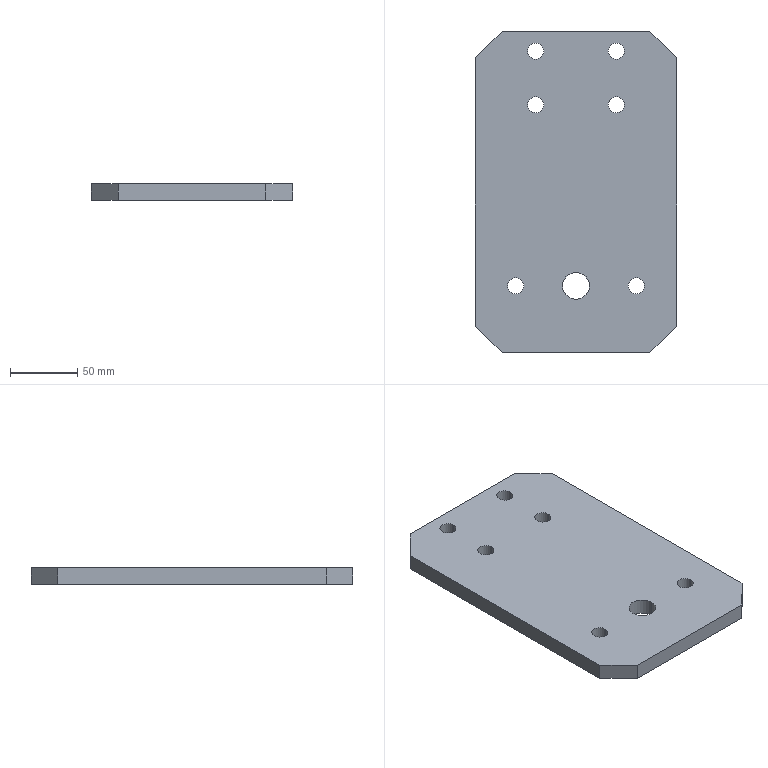Part | STEP file | Connecting plate | 1 solid | 24 faces | box 150 x 240 x 12 mm | volume 410487 mm3 | cylinder 14 | plane 10 | commonest cylinder face diameters 12 x12 20 x2
STEP:
#1=CARTESIAN_POINT('',(-24.923,-107.441,12.));
#2=VERTEX_POINT('',#1);
#3=CARTESIAN_POINT('',(-36.923,-107.441,12.));
#4=VERTEX_POINT('',#3);
#5=CARTESIAN_POINT('',(-30.923,-107.441,12.));
#6=DIRECTION('',(0.,0.,-1.));
#7=DIRECTION('',(-1.,0.,0.));
#8=AXIS2_PLACEMENT_3D('',#5,#6,#7);
#9=CIRCLE('',#8,6.);
#10=EDGE_CURVE('',#2,#4,#9,.T.);
#11=ORIENTED_EDGE('',*,*,#10,.F.);
#12=CARTESIAN_POINT('',(-24.923,-107.441,0.));
#13=VERTEX_POINT('',#12);
#14=CARTESIAN_POINT('',(-24.923,-107.441,12.));
#15=DIRECTION('',(0.,0.,-1.));
#16=VECTOR('',#15,1000.);
#17=LINE('',#14,#16);
#18=EDGE_CURVE('',#2,#13,#17,.T.);
#19=ORIENTED_EDGE('',*,*,#18,.T.);
#20=CARTESIAN_POINT('',(-36.923,-107.441,0.));
#21=VERTEX_POINT('',#20);
#22=CARTESIAN_POINT('',(-30.923,-107.441,0.));
#23=DIRECTION('',(0.,0.,-1.));
#24=DIRECTION('',(-1.,0.,0.));
#25=AXIS2_PLACEMENT_3D('',#22,#23,#24);
#26=CIRCLE('',#25,6.);
#27=EDGE_CURVE('',#13,#21,#26,.T.);
#28=ORIENTED_EDGE('',*,*,#27,.T.);
#29=CARTESIAN_POINT('',(-36.923,-107.441,12.));
#30=DIRECTION('',(0.,0.,-1.));
#31=VECTOR('',#30,1000.);
#32=LINE('',#29,#31);
#33=EDGE_CURVE('',#4,#21,#32,.T.);
#34=ORIENTED_EDGE('',*,*,#33,.F.);
#35=EDGE_LOOP('',(#11,#19,#28,#34));
#36=FACE_OUTER_BOUND('',#35,.T.);
#37=CARTESIAN_POINT('',(-30.923,-107.441,12.));
#38=DIRECTION('',(0.,0.,-1.));
#39=DIRECTION('',(-1.,0.,0.));
#40=AXIS2_PLACEMENT_3D('',#37,#38,#39);
#41=CYLINDRICAL_SURFACE('',#40,6.);
#42=ADVANCED_FACE('',(#36),#41,.F.);
#43=CARTESIAN_POINT('',(24.077,-107.441,12.));
#44=VERTEX_POINT('',#43);
#45=CARTESIAN_POINT('',(4.077,-107.441,12.));
#46=VERTEX_POINT('',#45);
#47=CARTESIAN_POINT('',(14.077,-107.441,12.));
#48=DIRECTION('',(0.,0.,-1.));
#49=DIRECTION('',(-1.,0.,0.));
#50=AXIS2_PLACEMENT_3D('',#47,#48,#49);
#51=CIRCLE('',#50,10.);
#52=EDGE_CURVE('',#44,#46,#51,.T.);
#53=ORIENTED_EDGE('',*,*,#52,.F.);
#54=CARTESIAN_POINT('',(24.077,-107.441,0.));
#55=VERTEX_POINT('',#54);
#56=CARTESIAN_POINT('',(24.077,-107.441,12.));
#57=DIRECTION('',(0.,0.,-1.));
#58=VECTOR('',#57,1000.);
#59=LINE('',#56,#58);
#60=EDGE_CURVE('',#44,#55,#59,.T.);
#61=ORIENTED_EDGE('',*,*,#60,.T.);
#62=CARTESIAN_POINT('',(4.077,-107.441,0.));
#63=VERTEX_POINT('',#62);
#64=CARTESIAN_POINT('',(14.077,-107.441,0.));
#65=DIRECTION('',(0.,0.,-1.));
#66=DIRECTION('',(-1.,0.,0.));
#67=AXIS2_PLACEMENT_3D('',#64,#65,#66);
#68=CIRCLE('',#67,10.);
#69=EDGE_CURVE('',#55,#63,#68,.T.);
#70=ORIENTED_EDGE('',*,*,#69,.T.);
#71=CARTESIAN_POINT('',(4.077,-107.441,12.));
#72=DIRECTION('',(0.,0.,-1.));
#73=VECTOR('',#72,1000.);
#74=LINE('',#71,#73);
#75=EDGE_CURVE('',#46,#63,#74,.T.);
#76=ORIENTED_EDGE('',*,*,#75,.F.);
#77=EDGE_LOOP('',(#53,#61,#70,#76));
#78=FACE_OUTER_BOUND('',#77,.T.);
#79=CARTESIAN_POINT('',(14.077,-107.441,12.));
#80=DIRECTION('',(0.,0.,-1.));
#81=DIRECTION('',(-1.,0.,0.));
#82=AXIS2_PLACEMENT_3D('',#79,#80,#81);
#83=CYLINDRICAL_SURFACE('',#82,10.);
#84=ADVANCED_FACE('',(#78),#83,.F.);
#85=CARTESIAN_POINT('',(50.077,27.559,12.));
#86=VERTEX_POINT('',#85);
#87=CARTESIAN_POINT('',(38.077,27.559,12.));
#88=VERTEX_POINT('',#87);
#89=CARTESIAN_POINT('',(44.077,27.559,12.));
#90=DIRECTION('',(0.,0.,-1.));
#91=DIRECTION('',(-1.,0.,0.));
#92=AXIS2_PLACEMENT_3D('',#89,#90,#91);
#93=CIRCLE('',#92,6.);
#94=EDGE_CURVE('',#86,#88,#93,.T.);
#95=ORIENTED_EDGE('',*,*,#94,.F.);
#96=CARTESIAN_POINT('',(50.077,27.559,0.));
#97=VERTEX_POINT('',#96);
#98=CARTESIAN_POINT('',(50.077,27.559,12.));
#99=DIRECTION('',(0.,0.,-1.));
#100=VECTOR('',#99,1000.);
#101=LINE('',#98,#100);
#102=EDGE_CURVE('',#86,#97,#101,.T.);
#103=ORIENTED_EDGE('',*,*,#102,.T.);
#104=CARTESIAN_POINT('',(38.077,27.559,0.));
#105=VERTEX_POINT('',#104);
#106=CARTESIAN_POINT('',(44.077,27.559,0.));
#107=DIRECTION('',(0.,0.,-1.));
#108=DIRECTION('',(-1.,0.,0.));
#109=AXIS2_PLACEMENT_3D('',#106,#107,#108);
#110=CIRCLE('',#109,6.);
#111=EDGE_CURVE('',#97,#105,#110,.T.);
#112=ORIENTED_EDGE('',*,*,#111,.T.);
#113=CARTESIAN_POINT('',(38.077,27.559,12.));
#114=DIRECTION('',(0.,0.,-1.));
#115=VECTOR('',#114,1000.);
#116=LINE('',#113,#115);
#117=EDGE_CURVE('',#88,#105,#116,.T.);
#118=ORIENTED_EDGE('',*,*,#117,.F.);
#119=EDGE_LOOP('',(#95,#103,#112,#118));
#120=FACE_OUTER_BOUND('',#119,.T.);
#121=CARTESIAN_POINT('',(44.077,27.559,12.));
#122=DIRECTION('',(0.,0.,-1.));
#123=DIRECTION('',(-1.,0.,0.));
#124=AXIS2_PLACEMENT_3D('',#121,#122,#123);
#125=CYLINDRICAL_SURFACE('',#124,6.);
#126=ADVANCED_FACE('',(#120),#125,.F.);
#127=CARTESIAN_POINT('',(-9.923,67.559,12.));
#128=VERTEX_POINT('',#127);
#129=CARTESIAN_POINT('',(-21.923,67.559,12.));
#130=VERTEX_POINT('',#129);
#131=CARTESIAN_POINT('',(-15.923,67.559,12.));
#132=DIRECTION('',(0.,0.,-1.));
#133=DIRECTION('',(-1.,0.,0.));
#134=AXIS2_PLACEMENT_3D('',#131,#132,#133);
#135=CIRCLE('',#134,6.);
#136=EDGE_CURVE('',#128,#130,#135,.T.);
#137=ORIENTED_EDGE('',*,*,#136,.F.);
#138=CARTESIAN_POINT('',(-9.923,67.559,0.));
#139=VERTEX_POINT('',#138);
#140=CARTESIAN_POINT('',(-9.923,67.559,12.));
#141=DIRECTION('',(0.,0.,-1.));
#142=VECTOR('',#141,1000.);
#143=LINE('',#140,#142);
#144=EDGE_CURVE('',#128,#139,#143,.T.);
#145=ORIENTED_EDGE('',*,*,#144,.T.);
#146=CARTESIAN_POINT('',(-21.923,67.559,0.));
#147=VERTEX_POINT('',#146);
#148=CARTESIAN_POINT('',(-15.923,67.559,0.));
#149=DIRECTION('',(0.,0.,-1.));
#150=DIRECTION('',(-1.,0.,0.));
#151=AXIS2_PLACEMENT_3D('',#148,#149,#150);
#152=CIRCLE('',#151,6.);
#153=EDGE_CURVE('',#139,#147,#152,.T.);
#154=ORIENTED_EDGE('',*,*,#153,.T.);
#155=CARTESIAN_POINT('',(-21.923,67.559,12.));
#156=DIRECTION('',(0.,0.,-1.));
#157=VECTOR('',#156,1000.);
#158=LINE('',#155,#157);
#159=EDGE_CURVE('',#130,#147,#158,.T.);
#160=ORIENTED_EDGE('',*,*,#159,.F.);
#161=EDGE_LOOP('',(#137,#145,#154,#160));
#162=FACE_OUTER_BOUND('',#161,.T.);
#163=CARTESIAN_POINT('',(-15.923,67.559,12.));
#164=DIRECTION('',(0.,0.,-1.));
#165=DIRECTION('',(-1.,0.,0.));
#166=AXIS2_PLACEMENT_3D('',#163,#164,#165);
#167=CYLINDRICAL_SURFACE('',#166,6.);
#168=ADVANCED_FACE('',(#162),#167,.F.);
#169=CARTESIAN_POINT('',(50.077,67.559,12.));
#170=VERTEX_POINT('',#169);
#171=CARTESIAN_POINT('',(38.077,67.559,12.));
#172=VERTEX_POINT('',#171);
#173=CARTESIAN_POINT('',(44.077,67.559,12.));
#174=DIRECTION('',(0.,0.,-1.));
#175=DIRECTION('',(-1.,0.,0.));
#176=AXIS2_PLACEMENT_3D('',#173,#174,#175);
#177=CIRCLE('',#176,6.);
#178=EDGE_CURVE('',#170,#172,#177,.T.);
#179=ORIENTED_EDGE('',*,*,#178,.F.);
#180=CARTESIAN_POINT('',(50.077,67.559,0.));
#181=VERTEX_POINT('',#180);
#182=CARTESIAN_POINT('',(50.077,67.559,12.));
#183=DIRECTION('',(0.,0.,-1.));
#184=VECTOR('',#183,1000.);
#185=LINE('',#182,#184);
#186=EDGE_CURVE('',#170,#181,#185,.T.);
#187=ORIENTED_EDGE('',*,*,#186,.T.);
#188=CARTESIAN_POINT('',(38.077,67.559,0.));
#189=VERTEX_POINT('',#188);
#190=CARTESIAN_POINT('',(44.077,67.559,0.));
#191=DIRECTION('',(0.,0.,-1.));
#192=DIRECTION('',(-1.,0.,0.));
#193=AXIS2_PLACEMENT_3D('',#190,#191,#192);
#194=CIRCLE('',#193,6.);
#195=EDGE_CURVE('',#181,#189,#194,.T.);
#196=ORIENTED_EDGE('',*,*,#195,.T.);
#197=CARTESIAN_POINT('',(38.077,67.559,12.));
#198=DIRECTION('',(0.,0.,-1.));
#199=VECTOR('',#198,1000.);
#200=LINE('',#197,#199);
#201=EDGE_CURVE('',#172,#189,#200,.T.);
#202=ORIENTED_EDGE('',*,*,#201,.F.);
#203=EDGE_LOOP('',(#179,#187,#196,#202));
#204=FACE_OUTER_BOUND('',#203,.T.);
#205=CARTESIAN_POINT('',(44.077,67.559,12.));
#206=DIRECTION('',(0.,0.,-1.));
#207=DIRECTION('',(-1.,0.,0.));
#208=AXIS2_PLACEMENT_3D('',#205,#206,#207);
#209=CYLINDRICAL_SURFACE('',#208,6.);
#210=ADVANCED_FACE('',(#204),#209,.F.);
#211=CARTESIAN_POINT('',(-9.923,27.559,12.));
#212=VERTEX_POINT('',#211);
#213=CARTESIAN_POINT('',(-21.923,27.559,12.));
#214=VERTEX_POINT('',#213);
#215=CARTESIAN_POINT('',(-15.923,27.559,12.));
#216=DIRECTION('',(0.,0.,-1.));
#217=DIRECTION('',(-1.,0.,0.));
#218=AXIS2_PLACEMENT_3D('',#215,#216,#217);
#219=CIRCLE('',#218,6.);
#220=EDGE_CURVE('',#212,#214,#219,.T.);
#221=ORIENTED_EDGE('',*,*,#220,.F.);
#222=CARTESIAN_POINT('',(-9.923,27.559,0.));
#223=VERTEX_POINT('',#222);
#224=CARTESIAN_POINT('',(-9.923,27.559,12.));
#225=DIRECTION('',(0.,0.,-1.));
#226=VECTOR('',#225,1000.);
#227=LINE('',#224,#226);
#228=EDGE_CURVE('',#212,#223,#227,.T.);
#229=ORIENTED_EDGE('',*,*,#228,.T.);
#230=CARTESIAN_POINT('',(-21.923,27.559,0.));
#231=VERTEX_POINT('',#230);
#232=CARTESIAN_POINT('',(-15.923,27.559,0.));
#233=DIRECTION('',(0.,0.,-1.));
#234=DIRECTION('',(-1.,0.,0.));
#235=AXIS2_PLACEMENT_3D('',#232,#233,#234);
#236=CIRCLE('',#235,6.);
#237=EDGE_CURVE('',#223,#231,#236,.T.);
#238=ORIENTED_EDGE('',*,*,#237,.T.);
#239=CARTESIAN_POINT('',(-21.923,27.559,12.));
#240=DIRECTION('',(0.,0.,-1.));
#241=VECTOR('',#240,1000.);
#242=LINE('',#239,#241);
#243=EDGE_CURVE('',#214,#231,#242,.T.);
#244=ORIENTED_EDGE('',*,*,#243,.F.);
#245=EDGE_LOOP('',(#221,#229,#238,#244));
#246=FACE_OUTER_BOUND('',#245,.T.);
#247=CARTESIAN_POINT('',(-15.923,27.559,12.));
#248=DIRECTION('',(0.,0.,-1.));
#249=DIRECTION('',(-1.,0.,0.));
#250=AXIS2_PLACEMENT_3D('',#247,#248,#249);
#251=CYLINDRICAL_SURFACE('',#250,6.);
#252=ADVANCED_FACE('',(#246),#251,.F.);
#253=CARTESIAN_POINT('',(65.077,-107.441,12.));
#254=VERTEX_POINT('',#253);
#255=CARTESIAN_POINT('',(53.077,-107.441,12.));
#256=VERTEX_POINT('',#255);
#257=CARTESIAN_POINT('',(59.077,-107.441,12.));
#258=DIRECTION('',(0.,0.,-1.));
#259=DIRECTION('',(-1.,0.,0.));
#260=AXIS2_PLACEMENT_3D('',#257,#258,#259);
#261=CIRCLE('',#260,6.);
#262=EDGE_CURVE('',#254,#256,#261,.T.);
#263=ORIENTED_EDGE('',*,*,#262,.F.);
#264=CARTESIAN_POINT('',(65.077,-107.441,0.));
#265=VERTEX_POINT('',#264);
#266=CARTESIAN_POINT('',(65.077,-107.441,12.));
#267=DIRECTION('',(0.,0.,-1.));
#268=VECTOR('',#267,1000.);
#269=LINE('',#266,#268);
#270=EDGE_CURVE('',#254,#265,#269,.T.);
#271=ORIENTED_EDGE('',*,*,#270,.T.);
#272=CARTESIAN_POINT('',(53.077,-107.441,0.));
#273=VERTEX_POINT('',#272);
#274=CARTESIAN_POINT('',(59.077,-107.441,0.));
#275=DIRECTION('',(0.,0.,-1.));
#276=DIRECTION('',(-1.,0.,0.));
#277=AXIS2_PLACEMENT_3D('',#274,#275,#276);
#278=CIRCLE('',#277,6.);
#279=EDGE_CURVE('',#265,#273,#278,.T.);
#280=ORIENTED_EDGE('',*,*,#279,.T.);
#281=CARTESIAN_POINT('',(53.077,-107.441,12.));
#282=DIRECTION('',(0.,0.,-1.));
#283=VECTOR('',#282,1000.);
#284=LINE('',#281,#283);
#285=EDGE_CURVE('',#256,#273,#284,.T.);
#286=ORIENTED_EDGE('',*,*,#285,.F.);
#287=EDGE_LOOP('',(#263,#271,#280,#286));
#288=FACE_OUTER_BOUND('',#287,.T.);
#289=CARTESIAN_POINT('',(59.077,-107.441,12.));
#290=DIRECTION('',(0.,0.,-1.));
#291=DIRECTION('',(-1.,0.,0.));
#292=AXIS2_PLACEMENT_3D('',#289,#290,#291);
#293=CYLINDRICAL_SURFACE('',#292,6.);
#294=ADVANCED_FACE('',(#288),#293,.F.);
#295=CARTESIAN_POINT('',(-30.923,-107.441,0.));
#296=DIRECTION('',(0.,0.,-1.));
#297=DIRECTION('',(-1.,0.,0.));
#298=AXIS2_PLACEMENT_3D('',#295,#296,#297);
#299=CIRCLE('',#298,6.);
#300=EDGE_CURVE('',#21,#13,#299,.T.);
#301=ORIENTED_EDGE('',*,*,#300,.F.);
#302=ORIENTED_EDGE('',*,*,#27,.F.);
#303=EDGE_LOOP('',(#301,#302));
#304=FACE_BOUND('',#303,.T.);
#305=CARTESIAN_POINT('',(14.077,-107.441,0.));
#306=DIRECTION('',(0.,0.,-1.));
#307=DIRECTION('',(-1.,0.,0.));
#308=AXIS2_PLACEMENT_3D('',#305,#306,#307);
#309=CIRCLE('',#308,10.);
#310=EDGE_CURVE('',#63,#55,#309,.T.);
#311=ORIENTED_EDGE('',*,*,#310,.F.);
#312=ORIENTED_EDGE('',*,*,#69,.F.);
#313=EDGE_LOOP('',(#311,#312));
#314=FACE_BOUND('',#313,.T.);
#315=CARTESIAN_POINT('',(44.077,27.559,0.));
#316=DIRECTION('',(0.,0.,-1.));
#317=DIRECTION('',(-1.,0.,0.));
#318=AXIS2_PLACEMENT_3D('',#315,#316,#317);
#319=CIRCLE('',#318,6.);
#320=EDGE_CURVE('',#105,#97,#319,.T.);
#321=ORIENTED_EDGE('',*,*,#320,.F.);
#322=ORIENTED_EDGE('',*,*,#111,.F.);
#323=EDGE_LOOP('',(#321,#322));
#324=FACE_BOUND('',#323,.T.);
#325=CARTESIAN_POINT('',(-15.923,67.559,0.));
#326=DIRECTION('',(0.,0.,-1.));
#327=DIRECTION('',(-1.,0.,0.));
#328=AXIS2_PLACEMENT_3D('',#325,#326,#327);
#329=CIRCLE('',#328,6.);
#330=EDGE_CURVE('',#147,#139,#329,.T.);
#331=ORIENTED_EDGE('',*,*,#330,.F.);
#332=ORIENTED_EDGE('',*,*,#153,.F.);
#333=EDGE_LOOP('',(#331,#332));
#334=FACE_BOUND('',#333,.T.);
#335=CARTESIAN_POINT('',(89.077,62.559,0.));
#336=VERTEX_POINT('',#335);
#337=CARTESIAN_POINT('',(69.077,82.559,0.));
#338=VERTEX_POINT('',#337);
#339=CARTESIAN_POINT('',(89.077,62.559,0.));
#340=DIRECTION('',(-0.7071,0.7071,0.));
#341=VECTOR('',#340,1000.);
#342=LINE('',#339,#341);
#343=EDGE_CURVE('',#336,#338,#342,.T.);
#344=ORIENTED_EDGE('',*,*,#343,.F.);
#345=CARTESIAN_POINT('',(89.077,-137.441,0.));
#346=VERTEX_POINT('',#345);
#347=CARTESIAN_POINT('',(89.077,-157.441,0.));
#348=DIRECTION('',(0.,1.,0.));
#349=VECTOR('',#348,1000.);
#350=LINE('',#347,#349);
#351=EDGE_CURVE('',#346,#336,#350,.T.);
#352=ORIENTED_EDGE('',*,*,#351,.F.);
#353=CARTESIAN_POINT('',(69.077,-157.441,0.));
#354=VERTEX_POINT('',#353);
#355=CARTESIAN_POINT('',(69.077,-157.441,0.));
#356=DIRECTION('',(0.7071,0.7071,0.));
#357=VECTOR('',#356,1000.);
#358=LINE('',#355,#357);
#359=EDGE_CURVE('',#354,#346,#358,.T.);
#360=ORIENTED_EDGE('',*,*,#359,.F.);
#361=CARTESIAN_POINT('',(-40.923,-157.441,0.));
#362=VERTEX_POINT('',#361);
#363=CARTESIAN_POINT('',(-60.923,-157.441,0.));
#364=DIRECTION('',(1.,0.,0.));
#365=VECTOR('',#364,1000.);
#366=LINE('',#363,#365);
#367=EDGE_CURVE('',#362,#354,#366,.T.);
#368=ORIENTED_EDGE('',*,*,#367,.F.);
#369=CARTESIAN_POINT('',(-60.923,-137.441,0.));
#370=VERTEX_POINT('',#369);
#371=CARTESIAN_POINT('',(-60.923,-137.441,0.));
#372=DIRECTION('',(0.7071,-0.7071,0.));
#373=VECTOR('',#372,1000.);
#374=LINE('',#371,#373);
#375=EDGE_CURVE('',#370,#362,#374,.T.);
#376=ORIENTED_EDGE('',*,*,#375,.F.);
#377=CARTESIAN_POINT('',(-60.923,62.559,0.));
#378=VERTEX_POINT('',#377);
#379=CARTESIAN_POINT('',(-60.923,-157.441,0.));
#380=DIRECTION('',(0.,-1.,0.));
#381=VECTOR('',#380,1000.);
#382=LINE('',#379,#381);
#383=EDGE_CURVE('',#378,#370,#382,.T.);
#384=ORIENTED_EDGE('',*,*,#383,.F.);
#385=CARTESIAN_POINT('',(-40.923,82.559,0.));
#386=VERTEX_POINT('',#385);
#387=CARTESIAN_POINT('',(-40.923,82.559,0.));
#388=DIRECTION('',(-0.7071,-0.7071,0.));
#389=VECTOR('',#388,1000.);
#390=LINE('',#387,#389);
#391=EDGE_CURVE('',#386,#378,#390,.T.);
#392=ORIENTED_EDGE('',*,*,#391,.F.);
#393=CARTESIAN_POINT('',(-60.923,82.559,0.));
#394=DIRECTION('',(-1.,0.,0.));
#395=VECTOR('',#394,1000.);
#396=LINE('',#393,#395);
#397=EDGE_CURVE('',#338,#386,#396,.T.);
#398=ORIENTED_EDGE('',*,*,#397,.F.);
#399=EDGE_LOOP('',(#344,#352,#360,#368,#376,#384,#392,#398));
#400=FACE_OUTER_BOUND('',#399,.T.);
#401=CARTESIAN_POINT('',(44.077,67.559,0.));
#402=DIRECTION('',(0.,0.,-1.));
#403=DIRECTION('',(-1.,0.,0.));
#404=AXIS2_PLACEMENT_3D('',#401,#402,#403);
#405=CIRCLE('',#404,6.);
#406=EDGE_CURVE('',#189,#181,#405,.T.);
#407=ORIENTED_EDGE('',*,*,#406,.F.);
#408=ORIENTED_EDGE('',*,*,#195,.F.);
#409=EDGE_LOOP('',(#407,#408));
#410=FACE_BOUND('',#409,.T.);
#411=CARTESIAN_POINT('',(-15.923,27.559,0.));
#412=DIRECTION('',(0.,0.,-1.));
#413=DIRECTION('',(-1.,0.,0.));
#414=AXIS2_PLACEMENT_3D('',#411,#412,#413);
#415=CIRCLE('',#414,6.);
#416=EDGE_CURVE('',#231,#223,#415,.T.);
#417=ORIENTED_EDGE('',*,*,#416,.F.);
#418=ORIENTED_EDGE('',*,*,#237,.F.);
#419=EDGE_LOOP('',(#417,#418));
#420=FACE_BOUND('',#419,.T.);
#421=CARTESIAN_POINT('',(59.077,-107.441,0.));
#422=DIRECTION('',(0.,0.,-1.));
#423=DIRECTION('',(-1.,0.,0.));
#424=AXIS2_PLACEMENT_3D('',#421,#422,#423);
#425=CIRCLE('',#424,6.);
#426=EDGE_CURVE('',#273,#265,#425,.T.);
#427=ORIENTED_EDGE('',*,*,#426,.F.);
#428=ORIENTED_EDGE('',*,*,#279,.F.);
#429=EDGE_LOOP('',(#427,#428));
#430=FACE_BOUND('',#429,.T.);
#431=CARTESIAN_POINT('',(-60.923,-157.441,0.));
#432=DIRECTION('',(0.,0.,1.));
#433=DIRECTION('',(1.,0.,0.));
#434=AXIS2_PLACEMENT_3D('',#431,#432,#433);
#435=PLANE('',#434);
#436=ADVANCED_FACE('',(#304,#314,#324,#334,#400,#410,#420,#430),#435,.F.);
#437=ORIENTED_EDGE('',*,*,#18,.F.);
#438=CARTESIAN_POINT('',(-30.923,-107.441,12.));
#439=DIRECTION('',(0.,0.,-1.));
#440=DIRECTION('',(-1.,0.,0.));
#441=AXIS2_PLACEMENT_3D('',#438,#439,#440);
#442=CIRCLE('',#441,6.);
#443=EDGE_CURVE('',#4,#2,#442,.T.);
#444=ORIENTED_EDGE('',*,*,#443,.F.);
#445=ORIENTED_EDGE('',*,*,#33,.T.);
#446=ORIENTED_EDGE('',*,*,#300,.T.);
#447=EDGE_LOOP('',(#437,#444,#445,#446));
#448=FACE_OUTER_BOUND('',#447,.T.);
#449=CARTESIAN_POINT('',(-30.923,-107.441,12.));
#450=DIRECTION('',(0.,0.,-1.));
#451=DIRECTION('',(-1.,0.,0.));
#452=AXIS2_PLACEMENT_3D('',#449,#450,#451);
#453=CYLINDRICAL_SURFACE('',#452,6.);
#454=ADVANCED_FACE('',(#448),#453,.F.);
#455=ORIENTED_EDGE('',*,*,#60,.F.);
#456=CARTESIAN_POINT('',(14.077,-107.441,12.));
#457=DIRECTION('',(0.,0.,-1.));
#458=DIRECTION('',(-1.,0.,0.));
#459=AXIS2_PLACEMENT_3D('',#456,#457,#458);
#460=CIRCLE('',#459,10.);
#461=EDGE_CURVE('',#46,#44,#460,.T.);
#462=ORIENTED_EDGE('',*,*,#461,.F.);
#463=ORIENTED_EDGE('',*,*,#75,.T.);
#464=ORIENTED_EDGE('',*,*,#310,.T.);
#465=EDGE_LOOP('',(#455,#462,#463,#464));
#466=FACE_OUTER_BOUND('',#465,.T.);
#467=CARTESIAN_POINT('',(14.077,-107.441,12.));
#468=DIRECTION('',(0.,0.,-1.));
#469=DIRECTION('',(-1.,0.,0.));
#470=AXIS2_PLACEMENT_3D('',#467,#468,#469);
#471=CYLINDRICAL_SURFACE('',#470,10.);
#472=ADVANCED_FACE('',(#466),#471,.F.);
#473=ORIENTED_EDGE('',*,*,#102,.F.);
#474=CARTESIAN_POINT('',(44.077,27.559,12.));
#475=DIRECTION('',(0.,0.,-1.));
#476=DIRECTION('',(-1.,0.,0.));
#477=AXIS2_PLACEMENT_3D('',#474,#475,#476);
#478=CIRCLE('',#477,6.);
#479=EDGE_CURVE('',#88,#86,#478,.T.);
#480=ORIENTED_EDGE('',*,*,#479,.F.);
#481=ORIENTED_EDGE('',*,*,#117,.T.);
#482=ORIENTED_EDGE('',*,*,#320,.T.);
#483=EDGE_LOOP('',(#473,#480,#481,#482));
#484=FACE_OUTER_BOUND('',#483,.T.);
#485=CARTESIAN_POINT('',(44.077,27.559,12.));
#486=DIRECTION('',(0.,0.,-1.));
#487=DIRECTION('',(-1.,0.,0.));
#488=AXIS2_PLACEMENT_3D('',#485,#486,#487);
#489=CYLINDRICAL_SURFACE('',#488,6.);
#490=ADVANCED_FACE('',(#484),#489,.F.);
#491=ORIENTED_EDGE('',*,*,#144,.F.);
#492=CARTESIAN_POINT('',(-15.923,67.559,12.));
#493=DIRECTION('',(0.,0.,-1.));
#494=DIRECTION('',(-1.,0.,0.));
#495=AXIS2_PLACEMENT_3D('',#492,#493,#494);
#496=CIRCLE('',#495,6.);
#497=EDGE_CURVE('',#130,#128,#496,.T.);
#498=ORIENTED_EDGE('',*,*,#497,.F.);
#499=ORIENTED_EDGE('',*,*,#159,.T.);
#500=ORIENTED_EDGE('',*,*,#330,.T.);
#501=EDGE_LOOP('',(#491,#498,#499,#500));
#502=FACE_OUTER_BOUND('',#501,.T.);
#503=CARTESIAN_POINT('',(-15.923,67.559,12.));
#504=DIRECTION('',(0.,0.,-1.));
#505=DIRECTION('',(-1.,0.,0.));
#506=AXIS2_PLACEMENT_3D('',#503,#504,#505);
#507=CYLINDRICAL_SURFACE('',#506,6.);
#508=ADVANCED_FACE('',(#502),#507,.F.);
#509=CARTESIAN_POINT('',(69.077,82.559,12.));
#510=VERTEX_POINT('',#509);
#511=CARTESIAN_POINT('',(69.077,82.559,12.));
#512=DIRECTION('',(0.,0.,1.));
#513=VECTOR('',#512,1000.);
#514=LINE('',#511,#513);
#515=EDGE_CURVE('',#338,#510,#514,.T.);
#516=ORIENTED_EDGE('',*,*,#515,.F.);
#517=ORIENTED_EDGE('',*,*,#397,.T.);
#518=CARTESIAN_POINT('',(-40.923,82.559,12.));
#519=VERTEX_POINT('',#518);
#520=CARTESIAN_POINT('',(-40.923,82.559,12.));
#521=DIRECTION('',(0.,0.,-1.));
#522=VECTOR('',#521,1000.);
#523=LINE('',#520,#522);
#524=EDGE_CURVE('',#519,#386,#523,.T.);
#525=ORIENTED_EDGE('',*,*,#524,.F.);
#526=CARTESIAN_POINT('',(-60.923,82.559,12.));
#527=DIRECTION('',(-1.,0.,0.));
#528=VECTOR('',#527,1000.);
#529=LINE('',#526,#528);
#530=EDGE_CURVE('',#510,#519,#529,.T.);
#531=ORIENTED_EDGE('',*,*,#530,.F.);
#532=EDGE_LOOP('',(#516,#517,#525,#531));
#533=FACE_OUTER_BOUND('',#532,.T.);
#534=CARTESIAN_POINT('',(-60.923,82.559,12.));
#535=DIRECTION('',(0.,-1.,0.));
#536=DIRECTION('',(0.,0.,-1.));
#537=AXIS2_PLACEMENT_3D('',#534,#535,#536);
#538=PLANE('',#537);
#539=ADVANCED_FACE('',(#533),#538,.F.);
#540=CARTESIAN_POINT('',(89.077,62.559,12.));
#541=VERTEX_POINT('',#540);
#542=CARTESIAN_POINT('',(89.077,62.559,12.));
#543=DIRECTION('',(0.,0.,1.));
#544=VECTOR('',#543,1000.);
#545=LINE('',#542,#544);
#546=EDGE_CURVE('',#336,#541,#545,.T.);
#547=ORIENTED_EDGE('',*,*,#546,.F.);
#548=ORIENTED_EDGE('',*,*,#343,.T.);
#549=ORIENTED_EDGE('',*,*,#515,.T.);
#550=CARTESIAN_POINT('',(69.077,82.559,12.));
#551=DIRECTION('',(-0.7071,0.7071,0.));
#552=VECTOR('',#551,1000.);
#553=LINE('',#550,#552);
#554=EDGE_CURVE('',#541,#510,#553,.T.);
#555=ORIENTED_EDGE('',*,*,#554,.F.);
#556=EDGE_LOOP('',(#547,#548,#549,#555));
#557=FACE_OUTER_BOUND('',#556,.T.);
#558=CARTESIAN_POINT('',(69.077,82.559,12.));
#559=DIRECTION('',(-0.7071,-0.7071,0.));
#560=DIRECTION('',(0.7071,-0.7071,0.));
#561=AXIS2_PLACEMENT_3D('',#558,#559,#560);
#562=PLANE('',#561);
#563=ADVANCED_FACE('',(#557),#562,.F.);
#564=ORIENTED_EDGE('',*,*,#546,.T.);
#565=CARTESIAN_POINT('',(89.077,-137.441,12.));
#566=VERTEX_POINT('',#565);
#567=CARTESIAN_POINT('',(89.077,82.559,12.));
#568=DIRECTION('',(0.,1.,0.));
#569=VECTOR('',#568,1000.);
#570=LINE('',#567,#569);
#571=EDGE_CURVE('',#566,#541,#570,.T.);
#572=ORIENTED_EDGE('',*,*,#571,.F.);
#573=CARTESIAN_POINT('',(89.077,-137.441,12.));
#574=DIRECTION('',(0.,0.,1.));
#575=VECTOR('',#574,1000.);
#576=LINE('',#573,#575);
#577=EDGE_CURVE('',#346,#566,#576,.T.);
#578=ORIENTED_EDGE('',*,*,#577,.F.);
#579=ORIENTED_EDGE('',*,*,#351,.T.);
#580=EDGE_LOOP('',(#564,#572,#578,#579));
#581=FACE_OUTER_BOUND('',#580,.T.);
#582=CARTESIAN_POINT('',(89.077,82.559,12.));
#583=DIRECTION('',(-1.,0.,0.));
#584=DIRECTION('',(0.,-1.,0.));
#585=AXIS2_PLACEMENT_3D('',#582,#583,#584);
#586=PLANE('',#585);
#587=ADVANCED_FACE('',(#581),#586,.F.);
#588=CARTESIAN_POINT('',(69.077,-157.441,12.));
#589=VERTEX_POINT('',#588);
#590=CARTESIAN_POINT('',(69.077,-157.441,12.));
#591=DIRECTION('',(0.,0.,1.));
#592=VECTOR('',#591,1000.);
#593=LINE('',#590,#592);
#594=EDGE_CURVE('',#354,#589,#593,.T.);
#595=ORIENTED_EDGE('',*,*,#594,.F.);
#596=ORIENTED_EDGE('',*,*,#359,.T.);
#597=ORIENTED_EDGE('',*,*,#577,.T.);
#598=CARTESIAN_POINT('',(89.077,-137.441,12.));
#599=DIRECTION('',(0.7071,0.7071,0.));
#600=VECTOR('',#599,1000.);
#601=LINE('',#598,#600);
#602=EDGE_CURVE('',#589,#566,#601,.T.);
#603=ORIENTED_EDGE('',*,*,#602,.F.);
#604=EDGE_LOOP('',(#595,#596,#597,#603));
#605=FACE_OUTER_BOUND('',#604,.T.);
#606=CARTESIAN_POINT('',(89.077,-137.441,12.));
#607=DIRECTION('',(-0.7071,0.7071,0.));
#608=DIRECTION('',(-0.7071,-0.7071,0.));
#609=AXIS2_PLACEMENT_3D('',#606,#607,#608);
#610=PLANE('',#609);
#611=ADVANCED_FACE('',(#605),#610,.F.);
#612=ORIENTED_EDGE('',*,*,#594,.T.);
#613=CARTESIAN_POINT('',(-40.923,-157.441,12.));
#614=VERTEX_POINT('',#613);
#615=CARTESIAN_POINT('',(-60.923,-157.441,12.));
#616=DIRECTION('',(1.,0.,0.));
#617=VECTOR('',#616,1000.);
#618=LINE('',#615,#617);
#619=EDGE_CURVE('',#614,#589,#618,.T.);
#620=ORIENTED_EDGE('',*,*,#619,.F.);
#621=CARTESIAN_POINT('',(-40.923,-157.441,12.));
#622=DIRECTION('',(0.,0.,1.));
#623=VECTOR('',#622,1000.);
#624=LINE('',#621,#623);
#625=EDGE_CURVE('',#362,#614,#624,.T.);
#626=ORIENTED_EDGE('',*,*,#625,.F.);
#627=ORIENTED_EDGE('',*,*,#367,.T.);
#628=EDGE_LOOP('',(#612,#620,#626,#627));
#629=FACE_OUTER_BOUND('',#628,.T.);
#630=CARTESIAN_POINT('',(-60.923,-157.441,12.));
#631=DIRECTION('',(0.,1.,0.));
#632=DIRECTION('',(0.,0.,1.));
#633=AXIS2_PLACEMENT_3D('',#630,#631,#632);
#634=PLANE('',#633);
#635=ADVANCED_FACE('',(#629),#634,.F.);
#636=CARTESIAN_POINT('',(-60.923,-137.441,12.));
#637=VERTEX_POINT('',#636);
#638=CARTESIAN_POINT('',(-60.923,-137.441,12.));
#639=DIRECTION('',(0.,0.,1.));
#640=VECTOR('',#639,1000.);
#641=LINE('',#638,#640);
#642=EDGE_CURVE('',#370,#637,#641,.T.);
#643=ORIENTED_EDGE('',*,*,#642,.F.);
#644=ORIENTED_EDGE('',*,*,#375,.T.);
#645=ORIENTED_EDGE('',*,*,#625,.T.);
#646=CARTESIAN_POINT('',(-40.923,-157.441,12.));
#647=DIRECTION('',(0.7071,-0.7071,0.));
#648=VECTOR('',#647,1000.);
#649=LINE('',#646,#648);
#650=EDGE_CURVE('',#637,#614,#649,.T.);
#651=ORIENTED_EDGE('',*,*,#650,.F.);
#652=EDGE_LOOP('',(#643,#644,#645,#651));
#653=FACE_OUTER_BOUND('',#652,.T.);
#654=CARTESIAN_POINT('',(-40.923,-157.441,12.));
#655=DIRECTION('',(0.7071,0.7071,0.));
#656=DIRECTION('',(-0.7071,0.7071,0.));
#657=AXIS2_PLACEMENT_3D('',#654,#655,#656);
#658=PLANE('',#657);
#659=ADVANCED_FACE('',(#653),#658,.F.);
#660=CARTESIAN_POINT('',(-60.923,62.559,12.));
#661=VERTEX_POINT('',#660);
#662=CARTESIAN_POINT('',(-60.923,62.559,12.));
#663=DIRECTION('',(0.,0.,1.));
#664=VECTOR('',#663,1000.);
#665=LINE('',#662,#664);
#666=EDGE_CURVE('',#378,#661,#665,.T.);
#667=ORIENTED_EDGE('',*,*,#666,.F.);
#668=ORIENTED_EDGE('',*,*,#383,.T.);
#669=ORIENTED_EDGE('',*,*,#642,.T.);
#670=CARTESIAN_POINT('',(-60.923,82.559,12.));
#671=DIRECTION('',(0.,-1.,0.));
#672=VECTOR('',#671,1000.);
#673=LINE('',#670,#672);
#674=EDGE_CURVE('',#661,#637,#673,.T.);
#675=ORIENTED_EDGE('',*,*,#674,.F.);
#676=EDGE_LOOP('',(#667,#668,#669,#675));
#677=FACE_OUTER_BOUND('',#676,.T.);
#678=CARTESIAN_POINT('',(-60.923,82.559,12.));
#679=DIRECTION('',(1.,0.,0.));
#680=DIRECTION('',(0.,1.,0.));
#681=AXIS2_PLACEMENT_3D('',#678,#679,#680);
#682=PLANE('',#681);
#683=ADVANCED_FACE('',(#677),#682,.F.);
#684=ORIENTED_EDGE('',*,*,#524,.T.);
#685=ORIENTED_EDGE('',*,*,#391,.T.);
#686=ORIENTED_EDGE('',*,*,#666,.T.);
#687=CARTESIAN_POINT('',(-60.923,62.559,12.));
#688=DIRECTION('',(-0.7071,-0.7071,0.));
#689=VECTOR('',#688,1000.);
#690=LINE('',#687,#689);
#691=EDGE_CURVE('',#519,#661,#690,.T.);
#692=ORIENTED_EDGE('',*,*,#691,.F.);
#693=EDGE_LOOP('',(#684,#685,#686,#692));
#694=FACE_OUTER_BOUND('',#693,.T.);
#695=CARTESIAN_POINT('',(-60.923,62.559,12.));
#696=DIRECTION('',(0.7071,-0.7071,0.));
#697=DIRECTION('',(0.7071,0.7071,0.));
#698=AXIS2_PLACEMENT_3D('',#695,#696,#697);
#699=PLANE('',#698);
#700=ADVANCED_FACE('',(#694),#699,.F.);
#701=ORIENTED_EDGE('',*,*,#186,.F.);
#702=CARTESIAN_POINT('',(44.077,67.559,12.));
#703=DIRECTION('',(0.,0.,-1.));
#704=DIRECTION('',(-1.,0.,0.));
#705=AXIS2_PLACEMENT_3D('',#702,#703,#704);
#706=CIRCLE('',#705,6.);
#707=EDGE_CURVE('',#172,#170,#706,.T.);
#708=ORIENTED_EDGE('',*,*,#707,.F.);
#709=ORIENTED_EDGE('',*,*,#201,.T.);
#710=ORIENTED_EDGE('',*,*,#406,.T.);
#711=EDGE_LOOP('',(#701,#708,#709,#710));
#712=FACE_OUTER_BOUND('',#711,.T.);
#713=CARTESIAN_POINT('',(44.077,67.559,12.));
#714=DIRECTION('',(0.,0.,-1.));
#715=DIRECTION('',(-1.,0.,0.));
#716=AXIS2_PLACEMENT_3D('',#713,#714,#715);
#717=CYLINDRICAL_SURFACE('',#716,6.);
#718=ADVANCED_FACE('',(#712),#717,.F.);
#719=ORIENTED_EDGE('',*,*,#228,.F.);
#720=CARTESIAN_POINT('',(-15.923,27.559,12.));
#721=DIRECTION('',(0.,0.,-1.));
#722=DIRECTION('',(-1.,0.,0.));
#723=AXIS2_PLACEMENT_3D('',#720,#721,#722);
#724=CIRCLE('',#723,6.);
#725=EDGE_CURVE('',#214,#212,#724,.T.);
#726=ORIENTED_EDGE('',*,*,#725,.F.);
#727=ORIENTED_EDGE('',*,*,#243,.T.);
#728=ORIENTED_EDGE('',*,*,#416,.T.);
#729=EDGE_LOOP('',(#719,#726,#727,#728));
#730=FACE_OUTER_BOUND('',#729,.T.);
#731=CARTESIAN_POINT('',(-15.923,27.559,12.));
#732=DIRECTION('',(0.,0.,-1.));
#733=DIRECTION('',(-1.,0.,0.));
#734=AXIS2_PLACEMENT_3D('',#731,#732,#733);
#735=CYLINDRICAL_SURFACE('',#734,6.);
#736=ADVANCED_FACE('',(#730),#735,.F.);
#737=ORIENTED_EDGE('',*,*,#270,.F.);
#738=CARTESIAN_POINT('',(59.077,-107.441,12.));
#739=DIRECTION('',(0.,0.,-1.));
#740=DIRECTION('',(-1.,0.,0.));
#741=AXIS2_PLACEMENT_3D('',#738,#739,#740);
#742=CIRCLE('',#741,6.);
#743=EDGE_CURVE('',#256,#254,#742,.T.);
#744=ORIENTED_EDGE('',*,*,#743,.F.);
#745=ORIENTED_EDGE('',*,*,#285,.T.);
#746=ORIENTED_EDGE('',*,*,#426,.T.);
#747=EDGE_LOOP('',(#737,#744,#745,#746));
#748=FACE_OUTER_BOUND('',#747,.T.);
#749=CARTESIAN_POINT('',(59.077,-107.441,12.));
#750=DIRECTION('',(0.,0.,-1.));
#751=DIRECTION('',(-1.,0.,0.));
#752=AXIS2_PLACEMENT_3D('',#749,#750,#751);
#753=CYLINDRICAL_SURFACE('',#752,6.);
#754=ADVANCED_FACE('',(#748),#753,.F.);
#755=ORIENTED_EDGE('',*,*,#443,.T.);
#756=ORIENTED_EDGE('',*,*,#10,.T.);
#757=EDGE_LOOP('',(#755,#756));
#758=FACE_BOUND('',#757,.T.);
#759=ORIENTED_EDGE('',*,*,#461,.T.);
#760=ORIENTED_EDGE('',*,*,#52,.T.);
#761=EDGE_LOOP('',(#759,#760));
#762=FACE_BOUND('',#761,.T.);
#763=ORIENTED_EDGE('',*,*,#479,.T.);
#764=ORIENTED_EDGE('',*,*,#94,.T.);
#765=EDGE_LOOP('',(#763,#764));
#766=FACE_BOUND('',#765,.T.);
#767=ORIENTED_EDGE('',*,*,#497,.T.);
#768=ORIENTED_EDGE('',*,*,#136,.T.);
#769=EDGE_LOOP('',(#767,#768));
#770=FACE_BOUND('',#769,.T.);
#771=ORIENTED_EDGE('',*,*,#619,.T.);
#772=ORIENTED_EDGE('',*,*,#602,.T.);
#773=ORIENTED_EDGE('',*,*,#571,.T.);
#774=ORIENTED_EDGE('',*,*,#554,.T.);
#775=ORIENTED_EDGE('',*,*,#530,.T.);
#776=ORIENTED_EDGE('',*,*,#691,.T.);
#777=ORIENTED_EDGE('',*,*,#674,.T.);
#778=ORIENTED_EDGE('',*,*,#650,.T.);
#779=EDGE_LOOP('',(#771,#772,#773,#774,#775,#776,#777,#778));
#780=FACE_OUTER_BOUND('',#779,.T.);
#781=ORIENTED_EDGE('',*,*,#707,.T.);
#782=ORIENTED_EDGE('',*,*,#178,.T.);
#783=EDGE_LOOP('',(#781,#782));
#784=FACE_BOUND('',#783,.T.);
#785=ORIENTED_EDGE('',*,*,#725,.T.);
#786=ORIENTED_EDGE('',*,*,#220,.T.);
#787=EDGE_LOOP('',(#785,#786));
#788=FACE_BOUND('',#787,.T.);
#789=ORIENTED_EDGE('',*,*,#743,.T.);
#790=ORIENTED_EDGE('',*,*,#262,.T.);
#791=EDGE_LOOP('',(#789,#790));
#792=FACE_BOUND('',#791,.T.);
#793=CARTESIAN_POINT('',(-60.923,-157.441,12.));
#794=DIRECTION('',(0.,0.,1.));
#795=DIRECTION('',(1.,0.,0.));
#796=AXIS2_PLACEMENT_3D('',#793,#794,#795);
#797=PLANE('',#796);
#798=ADVANCED_FACE('',(#758,#762,#766,#770,#780,#784,#788,#792),#797,.T.);
#799=CLOSED_SHELL('',(#42,#84,#126,#168,#210,#252,#294,#436,#454,#472,#490,#508,#539,#563,#587,#611,#635,#659,#683,#700,#718,#736,#754,#798));
#800=MANIFOLD_SOLID_BREP('',#799);
#801=CARTESIAN_POINT('',(0.,0.,0.));
#802=DIRECTION('',(0.,0.,1.));
#803=DIRECTION('',(1.,0.,0.));
#804=AXIS2_PLACEMENT_3D('',#801,#802,#803);
#805=(LENGTH_UNIT()NAMED_UNIT(*)SI_UNIT(.MILLI.,.METRE.));
#806=UNCERTAINTY_MEASURE_WITH_UNIT(LENGTH_MEASURE(0.00001),#805,'','');
#807=(NAMED_UNIT(*)PLANE_ANGLE_UNIT()SI_UNIT($,.RADIAN.));
#808=(NAMED_UNIT(*)SI_UNIT($,.STERADIAN.)SOLID_ANGLE_UNIT());
#809=(GEOMETRIC_REPRESENTATION_CONTEXT(3)GLOBAL_UNCERTAINTY_ASSIGNED_CONTEXT((#806))GLOBAL_UNIT_ASSIGNED_CONTEXT((#805,#807,#808))REPRESENTATION_CONTEXT('',''));
#810=ADVANCED_BREP_SHAPE_REPRESENTATION('',(#800,#804),#809);